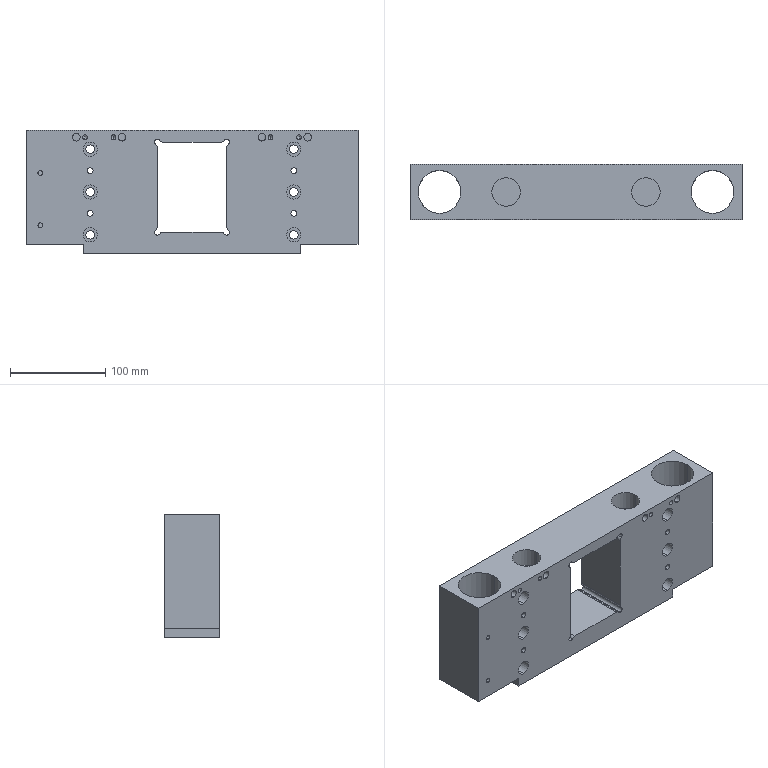Part | STEP file | 11-FG-SJ00811 | 1 solid | 146 faces | box 349 x 58 x 130 mm | volume 1666599 mm3 | cylinder 94 | cone 26 | plane 26 | commonest cylinder face diameters 5 x28 8 x16 6 x14 9 x12 15 x12 30 x8